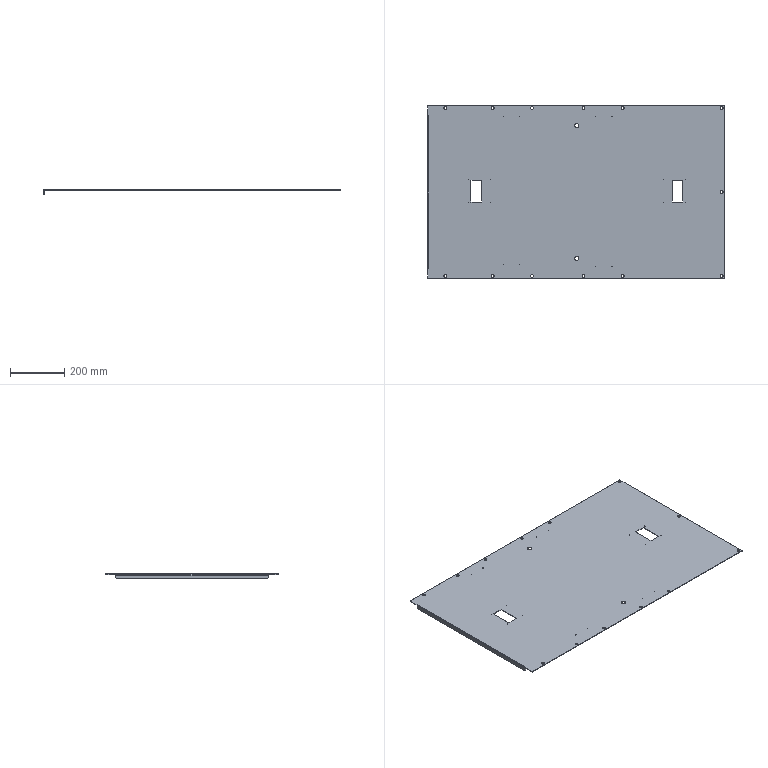Part | NX | features solid 2 | 1 solid | 94 faces | box 1095 x 640 x 15 mm | volume 1399226 mm3 | cylinder 70 | plane 24 | commonest cylinder face diameters 1 x32 10 x26 4 x7 15 x4 8 x1